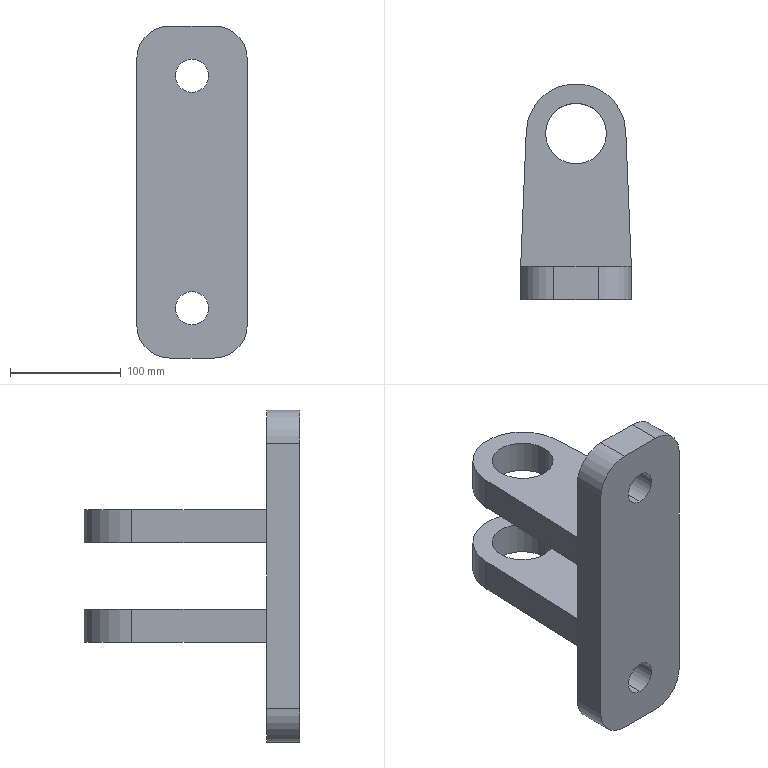Part | SolidWorks | features ICE 3, Extrusion 1, Fillet 1, MirrorPattern 1 | 1 solid | 30 faces | box 100 x 195 x 300 mm | volume 1566993 mm3 | plane 16 | cylinder 14 | commonest cylinder face diameters 30 x4 55 x4 60 x4 90 x2
STEP:
#1=CARTESIAN_POINT('',(0.,30.,90.));
#2=VERTEX_POINT('',#1);
#3=CARTESIAN_POINT('',(0.,30.,120.));
#4=VERTEX_POINT('',#3);
#5=CARTESIAN_POINT('',(0.,30.,105.));
#6=DIRECTION('',(0.,1.,0.));
#7=DIRECTION('',(0.,0.,-1.));
#8=AXIS2_PLACEMENT_3D('',#5,#6,#7);
#9=CIRCLE('',#8,15.);
#10=EDGE_CURVE('',#2,#4,#9,.T.);
#11=ORIENTED_EDGE('',*,*,#10,.T.);
#12=CARTESIAN_POINT('',(0.,0.,120.));
#13=VERTEX_POINT('',#12);
#14=CARTESIAN_POINT('',(0.,346.228,120.));
#15=DIRECTION('',(0.,-1.,0.));
#16=VECTOR('',#15,1000.);
#17=LINE('',#14,#16);
#18=EDGE_CURVE('',#4,#13,#17,.T.);
#19=ORIENTED_EDGE('',*,*,#18,.T.);
#20=CARTESIAN_POINT('',(0.,0.,90.));
#21=VERTEX_POINT('',#20);
#22=CARTESIAN_POINT('',(0.,0.,105.));
#23=DIRECTION('',(0.,-1.,0.));
#24=DIRECTION('',(0.,0.,1.));
#25=AXIS2_PLACEMENT_3D('',#22,#23,#24);
#26=CIRCLE('',#25,15.);
#27=EDGE_CURVE('',#13,#21,#26,.T.);
#28=ORIENTED_EDGE('',*,*,#27,.T.);
#29=CARTESIAN_POINT('',(0.,346.228,90.));
#30=DIRECTION('',(0.,-1.,0.));
#31=VECTOR('',#30,1000.);
#32=LINE('',#29,#31);
#33=EDGE_CURVE('',#2,#21,#32,.T.);
#34=ORIENTED_EDGE('',*,*,#33,.F.);
#35=EDGE_LOOP('',(#11,#19,#28,#34));
#36=FACE_OUTER_BOUND('',#35,.T.);
#37=CARTESIAN_POINT('',(0.,346.228,105.));
#38=DIRECTION('',(0.,-1.,0.));
#39=DIRECTION('',(0.,0.,-1.));
#40=AXIS2_PLACEMENT_3D('',#37,#38,#39);
#41=CYLINDRICAL_SURFACE('',#40,15.);
#42=ADVANCED_FACE('',(#36),#41,.F.);
#43=CARTESIAN_POINT('',(0.,30.,-120.));
#44=VERTEX_POINT('',#43);
#45=CARTESIAN_POINT('',(0.,30.,-90.));
#46=VERTEX_POINT('',#45);
#47=CARTESIAN_POINT('',(0.,30.,-105.));
#48=DIRECTION('',(0.,1.,0.));
#49=DIRECTION('',(0.,0.,-1.));
#50=AXIS2_PLACEMENT_3D('',#47,#48,#49);
#51=CIRCLE('',#50,15.);
#52=EDGE_CURVE('',#44,#46,#51,.T.);
#53=ORIENTED_EDGE('',*,*,#52,.T.);
#54=CARTESIAN_POINT('',(0.,0.,-90.));
#55=VERTEX_POINT('',#54);
#56=CARTESIAN_POINT('',(0.,346.228,-90.));
#57=DIRECTION('',(0.,-1.,0.));
#58=VECTOR('',#57,1000.);
#59=LINE('',#56,#58);
#60=EDGE_CURVE('',#46,#55,#59,.T.);
#61=ORIENTED_EDGE('',*,*,#60,.T.);
#62=CARTESIAN_POINT('',(0.,0.,-120.));
#63=VERTEX_POINT('',#62);
#64=CARTESIAN_POINT('',(0.,0.,-105.));
#65=DIRECTION('',(0.,-1.,0.));
#66=DIRECTION('',(0.,0.,-1.));
#67=AXIS2_PLACEMENT_3D('',#64,#65,#66);
#68=CIRCLE('',#67,15.);
#69=EDGE_CURVE('',#55,#63,#68,.T.);
#70=ORIENTED_EDGE('',*,*,#69,.T.);
#71=CARTESIAN_POINT('',(0.,346.228,-120.));
#72=DIRECTION('',(0.,-1.,0.));
#73=VECTOR('',#72,1000.);
#74=LINE('',#71,#73);
#75=EDGE_CURVE('',#44,#63,#74,.T.);
#76=ORIENTED_EDGE('',*,*,#75,.F.);
#77=EDGE_LOOP('',(#53,#61,#70,#76));
#78=FACE_OUTER_BOUND('',#77,.T.);
#79=CARTESIAN_POINT('',(0.,346.228,-105.));
#80=DIRECTION('',(0.,-1.,0.));
#81=DIRECTION('',(0.,0.,-1.));
#82=AXIS2_PLACEMENT_3D('',#79,#80,#81);
#83=CYLINDRICAL_SURFACE('',#82,15.);
#84=ADVANCED_FACE('',(#78),#83,.F.);
#85=CARTESIAN_POINT('',(-27.5,150.,-30.));
#86=VERTEX_POINT('',#85);
#87=CARTESIAN_POINT('',(27.5,150.,-30.));
#88=VERTEX_POINT('',#87);
#89=CARTESIAN_POINT('',(0.,150.,-30.));
#90=DIRECTION('',(0.,0.,1.));
#91=DIRECTION('',(1.,0.,0.));
#92=AXIS2_PLACEMENT_3D('',#89,#90,#91);
#93=CIRCLE('',#92,27.5);
#94=EDGE_CURVE('',#86,#88,#93,.T.);
#95=ORIENTED_EDGE('',*,*,#94,.T.);
#96=CARTESIAN_POINT('',(27.5,150.,-60.));
#97=VERTEX_POINT('',#96);
#98=CARTESIAN_POINT('',(27.5,150.,-30.));
#99=DIRECTION('',(0.,0.,-1.));
#100=VECTOR('',#99,1000.);
#101=LINE('',#98,#100);
#102=EDGE_CURVE('',#88,#97,#101,.T.);
#103=ORIENTED_EDGE('',*,*,#102,.T.);
#104=CARTESIAN_POINT('',(-27.5,150.,-60.));
#105=VERTEX_POINT('',#104);
#106=CARTESIAN_POINT('',(0.,150.,-60.));
#107=DIRECTION('',(0.,0.,1.));
#108=DIRECTION('',(1.,0.,0.));
#109=AXIS2_PLACEMENT_3D('',#106,#107,#108);
#110=CIRCLE('',#109,27.5);
#111=EDGE_CURVE('',#105,#97,#110,.T.);
#112=ORIENTED_EDGE('',*,*,#111,.F.);
#113=CARTESIAN_POINT('',(-27.5,150.,-30.));
#114=DIRECTION('',(0.,0.,-1.));
#115=VECTOR('',#114,1000.);
#116=LINE('',#113,#115);
#117=EDGE_CURVE('',#86,#105,#116,.T.);
#118=ORIENTED_EDGE('',*,*,#117,.F.);
#119=EDGE_LOOP('',(#95,#103,#112,#118));
#120=FACE_OUTER_BOUND('',#119,.T.);
#121=CARTESIAN_POINT('',(0.,150.,-30.));
#122=DIRECTION('',(0.,0.,-1.));
#123=DIRECTION('',(-1.,0.,0.));
#124=AXIS2_PLACEMENT_3D('',#121,#122,#123);
#125=CYLINDRICAL_SURFACE('',#124,27.5);
#126=ADVANCED_FACE('',(#120),#125,.F.);
#127=CARTESIAN_POINT('',(-27.5,150.,30.));
#128=VERTEX_POINT('',#127);
#129=CARTESIAN_POINT('',(27.5,150.,30.));
#130=VERTEX_POINT('',#129);
#131=CARTESIAN_POINT('',(0.,150.,30.));
#132=DIRECTION('',(0.,0.,1.));
#133=DIRECTION('',(1.,0.,0.));
#134=AXIS2_PLACEMENT_3D('',#131,#132,#133);
#135=CIRCLE('',#134,27.5);
#136=EDGE_CURVE('',#128,#130,#135,.T.);
#137=ORIENTED_EDGE('',*,*,#136,.F.);
#138=CARTESIAN_POINT('',(-27.5,150.,60.));
#139=VERTEX_POINT('',#138);
#140=CARTESIAN_POINT('',(-27.5,150.,30.));
#141=DIRECTION('',(0.,0.,1.));
#142=VECTOR('',#141,1000.);
#143=LINE('',#140,#142);
#144=EDGE_CURVE('',#128,#139,#143,.T.);
#145=ORIENTED_EDGE('',*,*,#144,.T.);
#146=CARTESIAN_POINT('',(27.5,150.,60.));
#147=VERTEX_POINT('',#146);
#148=CARTESIAN_POINT('',(0.,150.,60.));
#149=DIRECTION('',(0.,0.,1.));
#150=DIRECTION('',(1.,0.,0.));
#151=AXIS2_PLACEMENT_3D('',#148,#149,#150);
#152=CIRCLE('',#151,27.5);
#153=EDGE_CURVE('',#139,#147,#152,.T.);
#154=ORIENTED_EDGE('',*,*,#153,.T.);
#155=CARTESIAN_POINT('',(27.5,150.,30.));
#156=DIRECTION('',(0.,0.,1.));
#157=VECTOR('',#156,1000.);
#158=LINE('',#155,#157);
#159=EDGE_CURVE('',#130,#147,#158,.T.);
#160=ORIENTED_EDGE('',*,*,#159,.F.);
#161=EDGE_LOOP('',(#137,#145,#154,#160));
#162=FACE_OUTER_BOUND('',#161,.T.);
#163=CARTESIAN_POINT('',(0.,150.,30.));
#164=DIRECTION('',(0.,0.,1.));
#165=DIRECTION('',(1.,0.,0.));
#166=AXIS2_PLACEMENT_3D('',#163,#164,#165);
#167=CYLINDRICAL_SURFACE('',#166,27.5);
#168=ADVANCED_FACE('',(#162),#167,.F.);
#169=CARTESIAN_POINT('',(0.,150.,60.));
#170=DIRECTION('',(0.,0.,1.));
#171=DIRECTION('',(1.,0.,0.));
#172=AXIS2_PLACEMENT_3D('',#169,#170,#171);
#173=CIRCLE('',#172,27.5);
#174=EDGE_CURVE('',#147,#139,#173,.T.);
#175=ORIENTED_EDGE('',*,*,#174,.F.);
#176=ORIENTED_EDGE('',*,*,#153,.F.);
#177=EDGE_LOOP('',(#175,#176));
#178=FACE_BOUND('',#177,.T.);
#179=CARTESIAN_POINT('',(50.,30.,60.));
#180=VERTEX_POINT('',#179);
#181=CARTESIAN_POINT('',(-50.,30.,60.));
#182=VERTEX_POINT('',#181);
#183=CARTESIAN_POINT('',(-7.5,30.,60.));
#184=DIRECTION('',(-1.,0.,0.));
#185=VECTOR('',#184,1000.);
#186=LINE('',#183,#185);
#187=EDGE_CURVE('',#180,#182,#186,.T.);
#188=ORIENTED_EDGE('',*,*,#187,.F.);
#189=CARTESIAN_POINT('',(44.962,151.859,60.));
#190=VERTEX_POINT('',#189);
#191=CARTESIAN_POINT('',(44.962,151.859,60.));
#192=DIRECTION('',(-0.04131,0.9991,0.));
#193=VECTOR('',#192,1000.);
#194=LINE('',#191,#193);
#195=EDGE_CURVE('',#180,#190,#194,.T.);
#196=ORIENTED_EDGE('',*,*,#195,.T.);
#197=CARTESIAN_POINT('',(-44.962,151.859,60.));
#198=VERTEX_POINT('',#197);
#199=CARTESIAN_POINT('',(0.,150.,60.));
#200=DIRECTION('',(0.,0.,1.));
#201=DIRECTION('',(1.,0.,0.));
#202=AXIS2_PLACEMENT_3D('',#199,#200,#201);
#203=CIRCLE('',#202,45.);
#204=EDGE_CURVE('',#190,#198,#203,.T.);
#205=ORIENTED_EDGE('',*,*,#204,.T.);
#206=CARTESIAN_POINT('',(-44.962,151.859,60.));
#207=DIRECTION('',(-0.04131,-0.9991,0.));
#208=VECTOR('',#207,1000.);
#209=LINE('',#206,#208);
#210=EDGE_CURVE('',#198,#182,#209,.T.);
#211=ORIENTED_EDGE('',*,*,#210,.T.);
#212=EDGE_LOOP('',(#188,#196,#205,#211));
#213=FACE_OUTER_BOUND('',#212,.T.);
#214=CARTESIAN_POINT('',(-50.,30.,60.));
#215=DIRECTION('',(0.,0.,-1.));
#216=DIRECTION('',(-1.,0.,0.));
#217=AXIS2_PLACEMENT_3D('',#214,#215,#216);
#218=PLANE('',#217);
#219=ADVANCED_FACE('',(#178,#213),#218,.F.);
#220=ORIENTED_EDGE('',*,*,#111,.T.);
#221=CARTESIAN_POINT('',(0.,150.,-60.));
#222=DIRECTION('',(0.,0.,1.));
#223=DIRECTION('',(1.,0.,0.));
#224=AXIS2_PLACEMENT_3D('',#221,#222,#223);
#225=CIRCLE('',#224,27.5);
#226=EDGE_CURVE('',#97,#105,#225,.T.);
#227=ORIENTED_EDGE('',*,*,#226,.T.);
#228=EDGE_LOOP('',(#220,#227));
#229=FACE_BOUND('',#228,.T.);
#230=CARTESIAN_POINT('',(50.,30.,-60.));
#231=VERTEX_POINT('',#230);
#232=CARTESIAN_POINT('',(-50.,30.,-60.));
#233=VERTEX_POINT('',#232);
#234=CARTESIAN_POINT('',(-7.5,30.,-60.));
#235=DIRECTION('',(-1.,0.,0.));
#236=VECTOR('',#235,1000.);
#237=LINE('',#234,#236);
#238=EDGE_CURVE('',#231,#233,#237,.T.);
#239=ORIENTED_EDGE('',*,*,#238,.T.);
#240=CARTESIAN_POINT('',(-44.962,151.859,-60.));
#241=VERTEX_POINT('',#240);
#242=CARTESIAN_POINT('',(-44.962,151.859,-60.));
#243=DIRECTION('',(-0.04131,-0.9991,0.));
#244=VECTOR('',#243,1000.);
#245=LINE('',#242,#244);
#246=EDGE_CURVE('',#241,#233,#245,.T.);
#247=ORIENTED_EDGE('',*,*,#246,.F.);
#248=CARTESIAN_POINT('',(44.962,151.859,-60.));
#249=VERTEX_POINT('',#248);
#250=CARTESIAN_POINT('',(0.,150.,-60.));
#251=DIRECTION('',(0.,0.,1.));
#252=DIRECTION('',(1.,0.,0.));
#253=AXIS2_PLACEMENT_3D('',#250,#251,#252);
#254=CIRCLE('',#253,45.);
#255=EDGE_CURVE('',#249,#241,#254,.T.);
#256=ORIENTED_EDGE('',*,*,#255,.F.);
#257=CARTESIAN_POINT('',(44.962,151.859,-60.));
#258=DIRECTION('',(-0.04131,0.9991,0.));
#259=VECTOR('',#258,1000.);
#260=LINE('',#257,#259);
#261=EDGE_CURVE('',#231,#249,#260,.T.);
#262=ORIENTED_EDGE('',*,*,#261,.F.);
#263=EDGE_LOOP('',(#239,#247,#256,#262));
#264=FACE_OUTER_BOUND('',#263,.T.);
#265=CARTESIAN_POINT('',(-50.,30.,-60.));
#266=DIRECTION('',(0.,0.,1.));
#267=DIRECTION('',(1.,0.,0.));
#268=AXIS2_PLACEMENT_3D('',#265,#266,#267);
#269=PLANE('',#268);
#270=ADVANCED_FACE('',(#229,#264),#269,.F.);
#271=CARTESIAN_POINT('',(-50.,30.,-30.));
#272=VERTEX_POINT('',#271);
#273=CARTESIAN_POINT('',(50.,30.,-30.));
#274=VERTEX_POINT('',#273);
#275=CARTESIAN_POINT('',(-50.,30.,-30.));
#276=DIRECTION('',(1.,0.,0.));
#277=VECTOR('',#276,1000.);
#278=LINE('',#275,#277);
#279=EDGE_CURVE('',#272,#274,#278,.T.);
#280=ORIENTED_EDGE('',*,*,#279,.F.);
#281=CARTESIAN_POINT('',(-50.,30.,30.));
#282=VERTEX_POINT('',#281);
#283=CARTESIAN_POINT('',(-50.,30.,60.));
#284=DIRECTION('',(0.,0.,1.));
#285=VECTOR('',#284,1000.);
#286=LINE('',#283,#285);
#287=EDGE_CURVE('',#272,#282,#286,.T.);
#288=ORIENTED_EDGE('',*,*,#287,.T.);
#289=CARTESIAN_POINT('',(50.,30.,30.));
#290=VERTEX_POINT('',#289);
#291=CARTESIAN_POINT('',(-50.,30.,30.));
#292=DIRECTION('',(1.,0.,0.));
#293=VECTOR('',#292,1000.);
#294=LINE('',#291,#293);
#295=EDGE_CURVE('',#282,#290,#294,.T.);
#296=ORIENTED_EDGE('',*,*,#295,.T.);
#297=CARTESIAN_POINT('',(50.,30.,60.));
#298=DIRECTION('',(0.,0.,-1.));
#299=VECTOR('',#298,1000.);
#300=LINE('',#297,#299);
#301=EDGE_CURVE('',#290,#274,#300,.T.);
#302=ORIENTED_EDGE('',*,*,#301,.T.);
#303=EDGE_LOOP('',(#280,#288,#296,#302));
#304=FACE_OUTER_BOUND('',#303,.T.);
#305=CARTESIAN_POINT('',(0.,30.,0.));
#306=DIRECTION('',(0.,-1.,0.));
#307=DIRECTION('',(0.,0.,-1.));
#308=AXIS2_PLACEMENT_3D('',#305,#306,#307);
#309=PLANE('',#308);
#310=ADVANCED_FACE('',(#304),#309,.F.);
#311=CARTESIAN_POINT('',(50.,30.,120.));
#312=VERTEX_POINT('',#311);
#313=CARTESIAN_POINT('',(50.,30.,-150.));
#314=DIRECTION('',(0.,0.,-1.));
#315=VECTOR('',#314,1000.);
#316=LINE('',#313,#315);
#317=EDGE_CURVE('',#312,#180,#316,.T.);
#318=ORIENTED_EDGE('',*,*,#317,.F.);
#319=CARTESIAN_POINT('',(50.,0.,120.));
#320=VERTEX_POINT('',#319);
#321=CARTESIAN_POINT('',(50.,0.,120.));
#322=DIRECTION('',(0.,-1.,0.));
#323=VECTOR('',#322,1000.);
#324=LINE('',#321,#323);
#325=EDGE_CURVE('',#312,#320,#324,.T.);
#326=ORIENTED_EDGE('',*,*,#325,.T.);
#327=CARTESIAN_POINT('',(50.,0.,-120.));
#328=VERTEX_POINT('',#327);
#329=CARTESIAN_POINT('',(50.,0.,60.));
#330=DIRECTION('',(0.,0.,-1.));
#331=VECTOR('',#330,1000.);
#332=LINE('',#329,#331);
#333=EDGE_CURVE('',#320,#328,#332,.T.);
#334=ORIENTED_EDGE('',*,*,#333,.T.);
#335=CARTESIAN_POINT('',(50.,30.,-120.));
#336=VERTEX_POINT('',#335);
#337=CARTESIAN_POINT('',(50.,30.,-120.));
#338=DIRECTION('',(0.,1.,0.));
#339=VECTOR('',#338,1000.);
#340=LINE('',#337,#339);
#341=EDGE_CURVE('',#328,#336,#340,.T.);
#342=ORIENTED_EDGE('',*,*,#341,.T.);
#343=CARTESIAN_POINT('',(50.,30.,-150.));
#344=DIRECTION('',(0.,0.,-1.));
#345=VECTOR('',#344,1000.);
#346=LINE('',#343,#345);
#347=EDGE_CURVE('',#231,#336,#346,.T.);
#348=ORIENTED_EDGE('',*,*,#347,.F.);
#349=CARTESIAN_POINT('',(50.,30.,-30.));
#350=DIRECTION('',(0.,0.,-1.));
#351=VECTOR('',#350,1000.);
#352=LINE('',#349,#351);
#353=EDGE_CURVE('',#274,#231,#352,.T.);
#354=ORIENTED_EDGE('',*,*,#353,.F.);
#355=ORIENTED_EDGE('',*,*,#301,.F.);
#356=CARTESIAN_POINT('',(50.,30.,60.));
#357=DIRECTION('',(0.,0.,-1.));
#358=VECTOR('',#357,1000.);
#359=LINE('',#356,#358);
#360=EDGE_CURVE('',#180,#290,#359,.T.);
#361=ORIENTED_EDGE('',*,*,#360,.F.);
#362=EDGE_LOOP('',(#318,#326,#334,#342,#348,#354,#355,#361));
#363=FACE_OUTER_BOUND('',#362,.T.);
#364=CARTESIAN_POINT('',(50.,30.,60.));
#365=DIRECTION('',(-1.,0.,0.));
#366=DIRECTION('',(0.,0.,1.));
#367=AXIS2_PLACEMENT_3D('',#364,#365,#366);
#368=PLANE('',#367);
#369=ADVANCED_FACE('',(#363),#368,.F.);
#370=CARTESIAN_POINT('',(-50.,0.,-120.));
#371=VERTEX_POINT('',#370);
#372=CARTESIAN_POINT('',(-50.,0.,120.));
#373=VERTEX_POINT('',#372);
#374=CARTESIAN_POINT('',(-50.,0.,60.));
#375=DIRECTION('',(0.,0.,1.));
#376=VECTOR('',#375,1000.);
#377=LINE('',#374,#376);
#378=EDGE_CURVE('',#371,#373,#377,.T.);
#379=ORIENTED_EDGE('',*,*,#378,.T.);
#380=CARTESIAN_POINT('',(-50.,30.,120.));
#381=VERTEX_POINT('',#380);
#382=CARTESIAN_POINT('',(-50.,30.,120.));
#383=DIRECTION('',(0.,1.,0.));
#384=VECTOR('',#383,1000.);
#385=LINE('',#382,#384);
#386=EDGE_CURVE('',#373,#381,#385,.T.);
#387=ORIENTED_EDGE('',*,*,#386,.T.);
#388=CARTESIAN_POINT('',(-50.,30.,-150.));
#389=DIRECTION('',(0.,0.,1.));
#390=VECTOR('',#389,1000.);
#391=LINE('',#388,#390);
#392=EDGE_CURVE('',#182,#381,#391,.T.);
#393=ORIENTED_EDGE('',*,*,#392,.F.);
#394=CARTESIAN_POINT('',(-50.,30.,30.));
#395=DIRECTION('',(0.,0.,1.));
#396=VECTOR('',#395,1000.);
#397=LINE('',#394,#396);
#398=EDGE_CURVE('',#282,#182,#397,.T.);
#399=ORIENTED_EDGE('',*,*,#398,.F.);
#400=ORIENTED_EDGE('',*,*,#287,.F.);
#401=CARTESIAN_POINT('',(-50.,30.,60.));
#402=DIRECTION('',(0.,0.,1.));
#403=VECTOR('',#402,1000.);
#404=LINE('',#401,#403);
#405=EDGE_CURVE('',#233,#272,#404,.T.);
#406=ORIENTED_EDGE('',*,*,#405,.F.);
#407=CARTESIAN_POINT('',(-50.,30.,-120.));
#408=VERTEX_POINT('',#407);
#409=CARTESIAN_POINT('',(-50.,30.,-150.));
#410=DIRECTION('',(0.,0.,1.));
#411=VECTOR('',#410,1000.);
#412=LINE('',#409,#411);
#413=EDGE_CURVE('',#408,#233,#412,.T.);
#414=ORIENTED_EDGE('',*,*,#413,.F.);
#415=CARTESIAN_POINT('',(-50.,0.,-120.));
#416=DIRECTION('',(0.,-1.,0.));
#417=VECTOR('',#416,1000.);
#418=LINE('',#415,#417);
#419=EDGE_CURVE('',#408,#371,#418,.T.);
#420=ORIENTED_EDGE('',*,*,#419,.T.);
#421=EDGE_LOOP('',(#379,#387,#393,#399,#400,#406,#414,#420));
#422=FACE_OUTER_BOUND('',#421,.T.);
#423=CARTESIAN_POINT('',(-50.,30.,60.));
#424=DIRECTION('',(1.,0.,0.));
#425=DIRECTION('',(0.,0.,-1.));
#426=AXIS2_PLACEMENT_3D('',#423,#424,#425);
#427=PLANE('',#426);
#428=ADVANCED_FACE('',(#422),#427,.F.);
#429=ORIENTED_EDGE('',*,*,#333,.F.);
#430=CARTESIAN_POINT('',(20.,0.,150.));
#431=VERTEX_POINT('',#430);
#432=CARTESIAN_POINT('',(20.,0.,120.));
#433=DIRECTION('',(0.,-1.,0.));
#434=DIRECTION('',(0.,0.,-1.));
#435=AXIS2_PLACEMENT_3D('',#432,#433,#434);
#436=CIRCLE('',#435,30.);
#437=EDGE_CURVE('',#320,#431,#436,.T.);
#438=ORIENTED_EDGE('',*,*,#437,.T.);
#439=CARTESIAN_POINT('',(-20.,0.,150.));
#440=VERTEX_POINT('',#439);
#441=CARTESIAN_POINT('',(50.,0.,150.));
#442=DIRECTION('',(-1.,0.,0.));
#443=VECTOR('',#442,1000.);
#444=LINE('',#441,#443);
#445=EDGE_CURVE('',#431,#440,#444,.T.);
#446=ORIENTED_EDGE('',*,*,#445,.T.);
#447=CARTESIAN_POINT('',(-20.,0.,120.));
#448=DIRECTION('',(0.,-1.,0.));
#449=DIRECTION('',(0.,0.,-1.));
#450=AXIS2_PLACEMENT_3D('',#447,#448,#449);
#451=CIRCLE('',#450,30.);
#452=EDGE_CURVE('',#440,#373,#451,.T.);
#453=ORIENTED_EDGE('',*,*,#452,.T.);
#454=ORIENTED_EDGE('',*,*,#378,.F.);
#455=CARTESIAN_POINT('',(-20.,0.,-150.));
#456=VERTEX_POINT('',#455);
#457=CARTESIAN_POINT('',(-20.,0.,-120.));
#458=DIRECTION('',(0.,-1.,0.));
#459=DIRECTION('',(0.,0.,-1.));
#460=AXIS2_PLACEMENT_3D('',#457,#458,#459);
#461=CIRCLE('',#460,30.);
#462=EDGE_CURVE('',#371,#456,#461,.T.);
#463=ORIENTED_EDGE('',*,*,#462,.T.);
#464=CARTESIAN_POINT('',(20.,0.,-150.));
#465=VERTEX_POINT('',#464);
#466=CARTESIAN_POINT('',(50.,0.,-150.));
#467=DIRECTION('',(1.,0.,0.));
#468=VECTOR('',#467,1000.);
#469=LINE('',#466,#468);
#470=EDGE_CURVE('',#456,#465,#469,.T.);
#471=ORIENTED_EDGE('',*,*,#470,.T.);
#472=CARTESIAN_POINT('',(20.,0.,-120.));
#473=DIRECTION('',(0.,-1.,0.));
#474=DIRECTION('',(0.,0.,-1.));
#475=AXIS2_PLACEMENT_3D('',#472,#473,#474);
#476=CIRCLE('',#475,30.);
#477=EDGE_CURVE('',#465,#328,#476,.T.);
#478=ORIENTED_EDGE('',*,*,#477,.T.);
#479=EDGE_LOOP('',(#429,#438,#446,#453,#454,#463,#471,#478));
#480=FACE_OUTER_BOUND('',#479,.T.);
#481=CARTESIAN_POINT('',(0.,0.,105.));
#482=DIRECTION('',(0.,-1.,0.));
#483=DIRECTION('',(0.,0.,1.));
#484=AXIS2_PLACEMENT_3D('',#481,#482,#483);
#485=CIRCLE('',#484,15.);
#486=EDGE_CURVE('',#21,#13,#485,.T.);
#487=ORIENTED_EDGE('',*,*,#486,.F.);
#488=ORIENTED_EDGE('',*,*,#27,.F.);
#489=EDGE_LOOP('',(#487,#488));
#490=FACE_BOUND('',#489,.T.);
#491=CARTESIAN_POINT('',(0.,0.,-105.));
#492=DIRECTION('',(0.,-1.,0.));
#493=DIRECTION('',(0.,0.,-1.));
#494=AXIS2_PLACEMENT_3D('',#491,#492,#493);
#495=CIRCLE('',#494,15.);
#496=EDGE_CURVE('',#63,#55,#495,.T.);
#497=ORIENTED_EDGE('',*,*,#496,.F.);
#498=ORIENTED_EDGE('',*,*,#69,.F.);
#499=EDGE_LOOP('',(#497,#498));
#500=FACE_BOUND('',#499,.T.);
#501=CARTESIAN_POINT('',(0.,0.,0.));
#502=DIRECTION('',(0.,-1.,0.));
#503=DIRECTION('',(0.,0.,-1.));
#504=AXIS2_PLACEMENT_3D('',#501,#502,#503);
#505=PLANE('',#504);
#506=ADVANCED_FACE('',(#480,#490,#500),#505,.T.);
#507=ORIENTED_EDGE('',*,*,#204,.F.);
#508=CARTESIAN_POINT('',(44.962,151.859,30.));
#509=VERTEX_POINT('',#508);
#510=CARTESIAN_POINT('',(44.962,151.859,30.));
#511=DIRECTION('',(0.,0.,1.));
#512=VECTOR('',#511,1000.);
#513=LINE('',#510,#512);
#514=EDGE_CURVE('',#509,#190,#513,.T.);
#515=ORIENTED_EDGE('',*,*,#514,.F.);
#516=CARTESIAN_POINT('',(-44.962,151.859,30.));
#517=VERTEX_POINT('',#516);
#518=CARTESIAN_POINT('',(0.,150.,30.));
#519=DIRECTION('',(0.,0.,1.));
#520=DIRECTION('',(1.,0.,0.));
#521=AXIS2_PLACEMENT_3D('',#518,#519,#520);
#522=CIRCLE('',#521,45.);
#523=EDGE_CURVE('',#509,#517,#522,.T.);
#524=ORIENTED_EDGE('',*,*,#523,.T.);
#525=CARTESIAN_POINT('',(-44.962,151.859,30.));
#526=DIRECTION('',(0.,0.,1.));
#527=VECTOR('',#526,1000.);
#528=LINE('',#525,#527);
#529=EDGE_CURVE('',#517,#198,#528,.T.);
#530=ORIENTED_EDGE('',*,*,#529,.T.);
#531=EDGE_LOOP('',(#507,#515,#524,#530));
#532=FACE_OUTER_BOUND('',#531,.T.);
#533=CARTESIAN_POINT('',(0.,150.,30.));
#534=DIRECTION('',(0.,0.,1.));
#535=DIRECTION('',(1.,0.,0.));
#536=AXIS2_PLACEMENT_3D('',#533,#534,#535);
#537=CYLINDRICAL_SURFACE('',#536,45.);
#538=ADVANCED_FACE('',(#532),#537,.T.);
#539=ORIENTED_EDGE('',*,*,#195,.F.);
#540=ORIENTED_EDGE('',*,*,#360,.T.);
#541=CARTESIAN_POINT('',(44.962,151.859,30.));
#542=DIRECTION('',(-0.04131,0.9991,0.));
#543=VECTOR('',#542,1000.);
#544=LINE('',#541,#543);
#545=EDGE_CURVE('',#290,#509,#544,.T.);
#546=ORIENTED_EDGE('',*,*,#545,.T.);
#547=ORIENTED_EDGE('',*,*,#514,.T.);
#548=EDGE_LOOP('',(#539,#540,#546,#547));
#549=FACE_OUTER_BOUND('',#548,.T.);
#550=CARTESIAN_POINT('',(44.962,151.859,30.));
#551=DIRECTION('',(0.9991,0.04131,0.));
#552=DIRECTION('',(-0.04131,0.9991,0.));
#553=AXIS2_PLACEMENT_3D('',#550,#551,#552);
#554=PLANE('',#553);
#555=ADVANCED_FACE('',(#549),#554,.T.);
#556=ORIENTED_EDGE('',*,*,#210,.F.);
#557=ORIENTED_EDGE('',*,*,#529,.F.);
#558=CARTESIAN_POINT('',(-44.962,151.859,30.));
#559=DIRECTION('',(-0.04131,-0.9991,0.));
#560=VECTOR('',#559,1000.);
#561=LINE('',#558,#560);
#562=EDGE_CURVE('',#517,#282,#561,.T.);
#563=ORIENTED_EDGE('',*,*,#562,.T.);
#564=ORIENTED_EDGE('',*,*,#398,.T.);
#565=EDGE_LOOP('',(#556,#557,#563,#564));
#566=FACE_OUTER_BOUND('',#565,.T.);
#567=CARTESIAN_POINT('',(-44.962,151.859,30.));
#568=DIRECTION('',(-0.9991,0.04131,0.));
#569=DIRECTION('',(-0.04131,-0.9991,0.));
#570=AXIS2_PLACEMENT_3D('',#567,#568,#569);
#571=PLANE('',#570);
#572=ADVANCED_FACE('',(#566),#571,.T.);
#573=CARTESIAN_POINT('',(0.,150.,30.));
#574=DIRECTION('',(0.,0.,1.));
#575=DIRECTION('',(1.,0.,0.));
#576=AXIS2_PLACEMENT_3D('',#573,#574,#575);
#577=CIRCLE('',#576,27.5);
#578=EDGE_CURVE('',#130,#128,#577,.T.);
#579=ORIENTED_EDGE('',*,*,#578,.T.);
#580=ORIENTED_EDGE('',*,*,#136,.T.);
#581=EDGE_LOOP('',(#579,#580));
#582=FACE_BOUND('',#581,.T.);
#583=ORIENTED_EDGE('',*,*,#523,.F.);
#584=ORIENTED_EDGE('',*,*,#545,.F.);
#585=ORIENTED_EDGE('',*,*,#295,.F.);
#586=ORIENTED_EDGE('',*,*,#562,.F.);
#587=EDGE_LOOP('',(#583,#584,#585,#586));
#588=FACE_OUTER_BOUND('',#587,.T.);
#589=CARTESIAN_POINT('',(0.,150.,30.));
#590=DIRECTION('',(0.,0.,1.));
#591=DIRECTION('',(1.,0.,0.));
#592=AXIS2_PLACEMENT_3D('',#589,#590,#591);
#593=PLANE('',#592);
#594=ADVANCED_FACE('',(#582,#588),#593,.F.);
#595=ORIENTED_EDGE('',*,*,#144,.F.);
#596=ORIENTED_EDGE('',*,*,#578,.F.);
#597=ORIENTED_EDGE('',*,*,#159,.T.);
#598=ORIENTED_EDGE('',*,*,#174,.T.);
#599=EDGE_LOOP('',(#595,#596,#597,#598));
#600=FACE_OUTER_BOUND('',#599,.T.);
#601=CARTESIAN_POINT('',(0.,150.,30.));
#602=DIRECTION('',(0.,0.,1.));
#603=DIRECTION('',(1.,0.,0.));
#604=AXIS2_PLACEMENT_3D('',#601,#602,#603);
#605=CYLINDRICAL_SURFACE('',#604,27.5);
#606=ADVANCED_FACE('',(#600),#605,.F.);
#607=CARTESIAN_POINT('',(-20.,30.,150.));
#608=VERTEX_POINT('',#607);
#609=CARTESIAN_POINT('',(20.,30.,150.));
#610=VERTEX_POINT('',#609);
#611=CARTESIAN_POINT('',(50.,30.,150.));
#612=DIRECTION('',(1.,0.,0.));
#613=VECTOR('',#612,1000.);
#614=LINE('',#611,#613);
#615=EDGE_CURVE('',#608,#610,#614,.T.);
#616=ORIENTED_EDGE('',*,*,#615,.T.);
#617=CARTESIAN_POINT('',(20.,30.,120.));
#618=DIRECTION('',(0.,1.,0.));
#619=DIRECTION('',(0.,0.,-1.));
#620=AXIS2_PLACEMENT_3D('',#617,#618,#619);
#621=CIRCLE('',#620,30.);
#622=EDGE_CURVE('',#610,#312,#621,.T.);
#623=ORIENTED_EDGE('',*,*,#622,.T.);
#624=ORIENTED_EDGE('',*,*,#317,.T.);
#625=ORIENTED_EDGE('',*,*,#187,.T.);
#626=ORIENTED_EDGE('',*,*,#392,.T.);
#627=CARTESIAN_POINT('',(-20.,30.,120.));
#628=DIRECTION('',(0.,1.,0.));
#629=DIRECTION('',(0.,0.,-1.));
#630=AXIS2_PLACEMENT_3D('',#627,#628,#629);
#631=CIRCLE('',#630,30.);
#632=EDGE_CURVE('',#381,#608,#631,.T.);
#633=ORIENTED_EDGE('',*,*,#632,.T.);
#634=EDGE_LOOP('',(#616,#623,#624,#625,#626,#633));
#635=FACE_OUTER_BOUND('',#634,.T.);
#636=ORIENTED_EDGE('',*,*,#10,.F.);
#637=CARTESIAN_POINT('',(0.,30.,105.));
#638=DIRECTION('',(0.,1.,0.));
#639=DIRECTION('',(0.,0.,-1.));
#640=AXIS2_PLACEMENT_3D('',#637,#638,#639);
#641=CIRCLE('',#640,15.);
#642=EDGE_CURVE('',#4,#2,#641,.T.);
#643=ORIENTED_EDGE('',*,*,#642,.F.);
#644=EDGE_LOOP('',(#636,#643));
#645=FACE_BOUND('',#644,.T.);
#646=CARTESIAN_POINT('',(-7.5,30.,90.));
#647=DIRECTION('',(0.,-1.,0.));
#648=DIRECTION('',(0.,0.,-1.));
#649=AXIS2_PLACEMENT_3D('',#646,#647,#648);
#650=PLANE('',#649);
#651=ADVANCED_FACE('',(#635,#645),#650,.F.);
#652=CARTESIAN_POINT('',(44.962,151.859,-30.));
#653=VERTEX_POINT('',#652);
#654=CARTESIAN_POINT('',(-44.962,151.859,-30.));
#655=VERTEX_POINT('',#654);
#656=CARTESIAN_POINT('',(0.,150.,-30.));
#657=DIRECTION('',(0.,0.,1.));
#658=DIRECTION('',(1.,0.,0.));
#659=AXIS2_PLACEMENT_3D('',#656,#657,#658);
#660=CIRCLE('',#659,45.);
#661=EDGE_CURVE('',#653,#655,#660,.T.);
#662=ORIENTED_EDGE('',*,*,#661,.T.);
#663=CARTESIAN_POINT('',(-44.962,151.859,-30.));
#664=DIRECTION('',(-0.04131,-0.9991,0.));
#665=VECTOR('',#664,1000.);
#666=LINE('',#663,#665);
#667=EDGE_CURVE('',#655,#272,#666,.T.);
#668=ORIENTED_EDGE('',*,*,#667,.T.);
#669=ORIENTED_EDGE('',*,*,#279,.T.);
#670=CARTESIAN_POINT('',(44.962,151.859,-30.));
#671=DIRECTION('',(-0.04131,0.9991,0.));
#672=VECTOR('',#671,1000.);
#673=LINE('',#670,#672);
#674=EDGE_CURVE('',#274,#653,#673,.T.);
#675=ORIENTED_EDGE('',*,*,#674,.T.);
#676=EDGE_LOOP('',(#662,#668,#669,#675));
#677=FACE_OUTER_BOUND('',#676,.T.);
#678=ORIENTED_EDGE('',*,*,#94,.F.);
#679=CARTESIAN_POINT('',(0.,150.,-30.));
#680=DIRECTION('',(0.,0.,1.));
#681=DIRECTION('',(1.,0.,0.));
#682=AXIS2_PLACEMENT_3D('',#679,#680,#681);
#683=CIRCLE('',#682,27.5);
#684=EDGE_CURVE('',#88,#86,#683,.T.);
#685=ORIENTED_EDGE('',*,*,#684,.F.);
#686=EDGE_LOOP('',(#678,#685));
#687=FACE_BOUND('',#686,.T.);
#688=CARTESIAN_POINT('',(0.,150.,-30.));
#689=DIRECTION('',(0.,0.,-1.));
#690=DIRECTION('',(1.,0.,0.));
#691=AXIS2_PLACEMENT_3D('',#688,#689,#690);
#692=PLANE('',#691);
#693=ADVANCED_FACE('',(#677,#687),#692,.F.);
#694=ORIENTED_EDGE('',*,*,#255,.T.);
#695=CARTESIAN_POINT('',(-44.962,151.859,-30.));
#696=DIRECTION('',(0.,0.,-1.));
#697=VECTOR('',#696,1000.);
#698=LINE('',#695,#697);
#699=EDGE_CURVE('',#655,#241,#698,.T.);
#700=ORIENTED_EDGE('',*,*,#699,.F.);
#701=ORIENTED_EDGE('',*,*,#661,.F.);
#702=CARTESIAN_POINT('',(44.962,151.859,-30.));
#703=DIRECTION('',(0.,0.,-1.));
#704=VECTOR('',#703,1000.);
#705=LINE('',#702,#704);
#706=EDGE_CURVE('',#653,#249,#705,.T.);
#707=ORIENTED_EDGE('',*,*,#706,.T.);
#708=EDGE_LOOP('',(#694,#700,#701,#707));
#709=FACE_OUTER_BOUND('',#708,.T.);
#710=CARTESIAN_POINT('',(0.,150.,-30.));
#711=DIRECTION('',(0.,0.,-1.));
#712=DIRECTION('',(-1.,0.,0.));
#713=AXIS2_PLACEMENT_3D('',#710,#711,#712);
#714=CYLINDRICAL_SURFACE('',#713,45.);
#715=ADVANCED_FACE('',(#709),#714,.T.);
#716=ORIENTED_EDGE('',*,*,#246,.T.);
#717=ORIENTED_EDGE('',*,*,#405,.T.);
#718=ORIENTED_EDGE('',*,*,#667,.F.);
#719=ORIENTED_EDGE('',*,*,#699,.T.);
#720=EDGE_LOOP('',(#716,#717,#718,#719));
#721=FACE_OUTER_BOUND('',#720,.T.);
#722=CARTESIAN_POINT('',(-44.962,151.859,-30.));
#723=DIRECTION('',(0.9991,-0.04131,0.));
#724=DIRECTION('',(0.04131,0.9991,0.));
#725=AXIS2_PLACEMENT_3D('',#722,#723,#724);
#726=PLANE('',#725);
#727=ADVANCED_FACE('',(#721),#726,.F.);
#728=ORIENTED_EDGE('',*,*,#261,.T.);
#729=ORIENTED_EDGE('',*,*,#706,.F.);
#730=ORIENTED_EDGE('',*,*,#674,.F.);
#731=ORIENTED_EDGE('',*,*,#353,.T.);
#732=EDGE_LOOP('',(#728,#729,#730,#731));
#733=FACE_OUTER_BOUND('',#732,.T.);
#734=CARTESIAN_POINT('',(44.962,151.859,-30.));
#735=DIRECTION('',(-0.9991,-0.04131,0.));
#736=DIRECTION('',(0.04131,-0.9991,0.));
#737=AXIS2_PLACEMENT_3D('',#734,#735,#736);
#738=PLANE('',#737);
#739=ADVANCED_FACE('',(#733),#738,.F.);
#740=ORIENTED_EDGE('',*,*,#102,.F.);
#741=ORIENTED_EDGE('',*,*,#684,.T.);
#742=ORIENTED_EDGE('',*,*,#117,.T.);
#743=ORIENTED_EDGE('',*,*,#226,.F.);
#744=EDGE_LOOP('',(#740,#741,#742,#743));
#745=FACE_OUTER_BOUND('',#744,.T.);
#746=CARTESIAN_POINT('',(0.,150.,-30.));
#747=DIRECTION('',(0.,0.,-1.));
#748=DIRECTION('',(-1.,0.,0.));
#749=AXIS2_PLACEMENT_3D('',#746,#747,#748);
#750=CYLINDRICAL_SURFACE('',#749,27.5);
#751=ADVANCED_FACE('',(#745),#750,.F.);
#752=ORIENTED_EDGE('',*,*,#347,.T.);
#753=CARTESIAN_POINT('',(20.,30.,-150.));
#754=VERTEX_POINT('',#753);
#755=CARTESIAN_POINT('',(20.,30.,-120.));
#756=DIRECTION('',(0.,1.,0.));
#757=DIRECTION('',(0.,0.,1.));
#758=AXIS2_PLACEMENT_3D('',#755,#756,#757);
#759=CIRCLE('',#758,30.);
#760=EDGE_CURVE('',#336,#754,#759,.T.);
#761=ORIENTED_EDGE('',*,*,#760,.T.);
#762=CARTESIAN_POINT('',(-20.,30.,-150.));
#763=VERTEX_POINT('',#762);
#764=CARTESIAN_POINT('',(50.,30.,-150.));
#765=DIRECTION('',(-1.,0.,0.));
#766=VECTOR('',#765,1000.);
#767=LINE('',#764,#766);
#768=EDGE_CURVE('',#754,#763,#767,.T.);
#769=ORIENTED_EDGE('',*,*,#768,.T.);
#770=CARTESIAN_POINT('',(-20.,30.,-120.));
#771=DIRECTION('',(0.,1.,0.));
#772=DIRECTION('',(0.,0.,1.));
#773=AXIS2_PLACEMENT_3D('',#770,#771,#772);
#774=CIRCLE('',#773,30.);
#775=EDGE_CURVE('',#763,#408,#774,.T.);
#776=ORIENTED_EDGE('',*,*,#775,.T.);
#777=ORIENTED_EDGE('',*,*,#413,.T.);
#778=ORIENTED_EDGE('',*,*,#238,.F.);
#779=EDGE_LOOP('',(#752,#761,#769,#776,#777,#778));
#780=FACE_OUTER_BOUND('',#779,.T.);
#781=ORIENTED_EDGE('',*,*,#52,.F.);
#782=CARTESIAN_POINT('',(0.,30.,-105.));
#783=DIRECTION('',(0.,1.,0.));
#784=DIRECTION('',(0.,0.,-1.));
#785=AXIS2_PLACEMENT_3D('',#782,#783,#784);
#786=CIRCLE('',#785,15.);
#787=EDGE_CURVE('',#46,#44,#786,.T.);
#788=ORIENTED_EDGE('',*,*,#787,.F.);
#789=EDGE_LOOP('',(#781,#788));
#790=FACE_BOUND('',#789,.T.);
#791=CARTESIAN_POINT('',(-7.5,30.,-90.));
#792=DIRECTION('',(0.,1.,0.));
#793=DIRECTION('',(0.,0.,1.));
#794=AXIS2_PLACEMENT_3D('',#791,#792,#793);
#795=PLANE('',#794);
#796=ADVANCED_FACE('',(#780,#790),#795,.T.);
#797=ORIENTED_EDGE('',*,*,#768,.F.);
#798=CARTESIAN_POINT('',(20.,0.,-150.));
#799=DIRECTION('',(0.,-1.,0.));
#800=VECTOR('',#799,1000.);
#801=LINE('',#798,#800);
#802=EDGE_CURVE('',#754,#465,#801,.T.);
#803=ORIENTED_EDGE('',*,*,#802,.T.);
#804=ORIENTED_EDGE('',*,*,#470,.F.);
#805=CARTESIAN_POINT('',(-20.,30.,-150.));
#806=DIRECTION('',(0.,1.,0.));
#807=VECTOR('',#806,1000.);
#808=LINE('',#805,#807);
#809=EDGE_CURVE('',#456,#763,#808,.T.);
#810=ORIENTED_EDGE('',*,*,#809,.T.);
#811=EDGE_LOOP('',(#797,#803,#804,#810));
#812=FACE_OUTER_BOUND('',#811,.T.);
#813=CARTESIAN_POINT('',(50.,346.228,-150.));
#814=DIRECTION('',(0.,0.,-1.));
#815=DIRECTION('',(-1.,0.,0.));
#816=AXIS2_PLACEMENT_3D('',#813,#814,#815);
#817=PLANE('',#816);
#818=ADVANCED_FACE('',(#812),#817,.T.);
#819=ORIENTED_EDGE('',*,*,#60,.F.);
#820=ORIENTED_EDGE('',*,*,#787,.T.);
#821=ORIENTED_EDGE('',*,*,#75,.T.);
#822=ORIENTED_EDGE('',*,*,#496,.T.);
#823=EDGE_LOOP('',(#819,#820,#821,#822));
#824=FACE_OUTER_BOUND('',#823,.T.);
#825=CARTESIAN_POINT('',(0.,346.228,-105.));
#826=DIRECTION('',(0.,-1.,0.));
#827=DIRECTION('',(0.,0.,-1.));
#828=AXIS2_PLACEMENT_3D('',#825,#826,#827);
#829=CYLINDRICAL_SURFACE('',#828,15.);
#830=ADVANCED_FACE('',(#824),#829,.F.);
#831=ORIENTED_EDGE('',*,*,#445,.F.);
#832=CARTESIAN_POINT('',(20.,30.,150.));
#833=DIRECTION('',(0.,1.,0.));
#834=VECTOR('',#833,1000.);
#835=LINE('',#832,#834);
#836=EDGE_CURVE('',#431,#610,#835,.T.);
#837=ORIENTED_EDGE('',*,*,#836,.T.);
#838=ORIENTED_EDGE('',*,*,#615,.F.);
#839=CARTESIAN_POINT('',(-20.,0.,150.));
#840=DIRECTION('',(0.,-1.,0.));
#841=VECTOR('',#840,1000.);
#842=LINE('',#839,#841);
#843=EDGE_CURVE('',#608,#440,#842,.T.);
#844=ORIENTED_EDGE('',*,*,#843,.T.);
#845=EDGE_LOOP('',(#831,#837,#838,#844));
#846=FACE_OUTER_BOUND('',#845,.T.);
#847=CARTESIAN_POINT('',(50.,346.228,150.));
#848=DIRECTION('',(0.,0.,1.));
#849=DIRECTION('',(1.,0.,0.));
#850=AXIS2_PLACEMENT_3D('',#847,#848,#849);
#851=PLANE('',#850);
#852=ADVANCED_FACE('',(#846),#851,.T.);
#853=ORIENTED_EDGE('',*,*,#18,.F.);
#854=ORIENTED_EDGE('',*,*,#642,.T.);
#855=ORIENTED_EDGE('',*,*,#33,.T.);
#856=ORIENTED_EDGE('',*,*,#486,.T.);
#857=EDGE_LOOP('',(#853,#854,#855,#856));
#858=FACE_OUTER_BOUND('',#857,.T.);
#859=CARTESIAN_POINT('',(0.,346.228,105.));
#860=DIRECTION('',(0.,-1.,0.));
#861=DIRECTION('',(0.,0.,-1.));
#862=AXIS2_PLACEMENT_3D('',#859,#860,#861);
#863=CYLINDRICAL_SURFACE('',#862,15.);
#864=ADVANCED_FACE('',(#858),#863,.F.);
#865=ORIENTED_EDGE('',*,*,#622,.F.);
#866=ORIENTED_EDGE('',*,*,#836,.F.);
#867=ORIENTED_EDGE('',*,*,#437,.F.);
#868=ORIENTED_EDGE('',*,*,#325,.F.);
#869=EDGE_LOOP('',(#865,#866,#867,#868));
#870=FACE_OUTER_BOUND('',#869,.T.);
#871=CARTESIAN_POINT('',(20.,30.,120.));
#872=DIRECTION('',(0.,1.,0.));
#873=DIRECTION('',(0.,0.,1.));
#874=AXIS2_PLACEMENT_3D('',#871,#872,#873);
#875=CYLINDRICAL_SURFACE('',#874,30.);
#876=ADVANCED_FACE('',(#870),#875,.T.);
#877=ORIENTED_EDGE('',*,*,#632,.F.);
#878=ORIENTED_EDGE('',*,*,#386,.F.);
#879=ORIENTED_EDGE('',*,*,#452,.F.);
#880=ORIENTED_EDGE('',*,*,#843,.F.);
#881=EDGE_LOOP('',(#877,#878,#879,#880));
#882=FACE_OUTER_BOUND('',#881,.T.);
#883=CARTESIAN_POINT('',(-20.,346.228,120.));
#884=DIRECTION('',(0.,1.,0.));
#885=DIRECTION('',(0.,0.,1.));
#886=AXIS2_PLACEMENT_3D('',#883,#884,#885);
#887=CYLINDRICAL_SURFACE('',#886,30.);
#888=ADVANCED_FACE('',(#882),#887,.T.);
#889=ORIENTED_EDGE('',*,*,#760,.F.);
#890=ORIENTED_EDGE('',*,*,#341,.F.);
#891=ORIENTED_EDGE('',*,*,#477,.F.);
#892=ORIENTED_EDGE('',*,*,#802,.F.);
#893=EDGE_LOOP('',(#889,#890,#891,#892));
#894=FACE_OUTER_BOUND('',#893,.T.);
#895=CARTESIAN_POINT('',(20.,346.228,-120.));
#896=DIRECTION('',(0.,1.,0.));
#897=DIRECTION('',(0.,0.,1.));
#898=AXIS2_PLACEMENT_3D('',#895,#896,#897);
#899=CYLINDRICAL_SURFACE('',#898,30.);
#900=ADVANCED_FACE('',(#894),#899,.T.);
#901=ORIENTED_EDGE('',*,*,#775,.F.);
#902=ORIENTED_EDGE('',*,*,#809,.F.);
#903=ORIENTED_EDGE('',*,*,#462,.F.);
#904=ORIENTED_EDGE('',*,*,#419,.F.);
#905=EDGE_LOOP('',(#901,#902,#903,#904));
#906=FACE_OUTER_BOUND('',#905,.T.);
#907=CARTESIAN_POINT('',(-20.,30.,-120.));
#908=DIRECTION('',(0.,1.,0.));
#909=DIRECTION('',(0.,0.,1.));
#910=AXIS2_PLACEMENT_3D('',#907,#908,#909);
#911=CYLINDRICAL_SURFACE('',#910,30.);
#912=ADVANCED_FACE('',(#906),#911,.T.);
#913=CLOSED_SHELL('',(#42,#84,#126,#168,#219,#270,#310,#369,#428,#506,#538,#555,#572,#594,#606,#651,#693,#715,#727,#739,#751,#796,#818,#830,#852,#864,#876,#888,#900,#912));
#914=MANIFOLD_SOLID_BREP('',#913);
#915=CARTESIAN_POINT('',(0.,0.,0.));
#916=DIRECTION('',(0.,0.,1.));
#917=DIRECTION('',(1.,0.,0.));
#918=AXIS2_PLACEMENT_3D('',#915,#916,#917);
#919=(LENGTH_UNIT()NAMED_UNIT(*)SI_UNIT(.MILLI.,.METRE.));
#920=UNCERTAINTY_MEASURE_WITH_UNIT(LENGTH_MEASURE(0.00001),#919,'','');
#921=(NAMED_UNIT(*)PLANE_ANGLE_UNIT()SI_UNIT($,.RADIAN.));
#922=(NAMED_UNIT(*)SI_UNIT($,.STERADIAN.)SOLID_ANGLE_UNIT());
#923=(GEOMETRIC_REPRESENTATION_CONTEXT(3)GLOBAL_UNCERTAINTY_ASSIGNED_CONTEXT((#920))GLOBAL_UNIT_ASSIGNED_CONTEXT((#919,#921,#922))REPRESENTATION_CONTEXT('',''));
#924=ADVANCED_BREP_SHAPE_REPRESENTATION('',(#914,#918),#923);